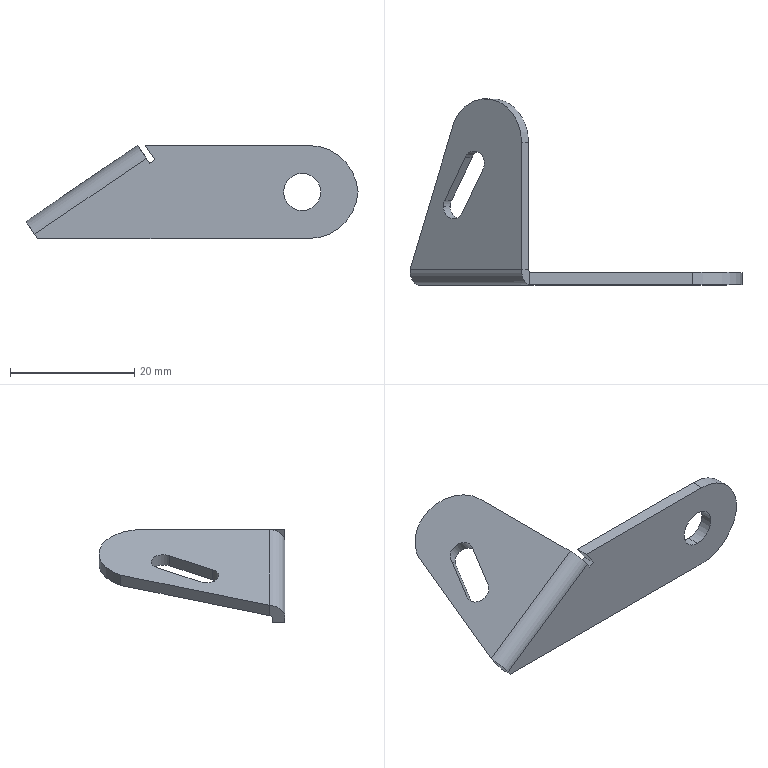Part | SolidWorks | features ICE 3, Cut 2, Fillet 2, EdgeFlange 1, FlatPattern 1, SMBaseFlange 1, SheetMetal 1 | 1 solid | 25 faces | box 53.504 x 30 x 15 mm | volume 2061 mm3 | plane 15 | cylinder 10 | commonest cylinder face diameters 4 x3 6 x2 16 x2 1 x1 5 x1 14 x1
STEP:
#1=CARTESIAN_POINT('',(-11.933,11.65,-0.9332));
#2=VERTEX_POINT('',#1);
#3=CARTESIAN_POINT('',(-12.155,10.65,-1.084));
#4=VERTEX_POINT('',#3);
#5=CARTESIAN_POINT('',(-10.501,10.65,0.04121));
#6=DIRECTION('',(-0.5626,0.,0.8267));
#7=DIRECTION('',(0.8267,0.,0.5626));
#8=AXIS2_PLACEMENT_3D('',#5,#6,#7);
#9=CIRCLE('',#8,2.);
#10=EDGE_CURVE('',#2,#4,#9,.T.);
#11=ORIENTED_EDGE('',*,*,#10,.T.);
#12=CARTESIAN_POINT('',(-11.03,10.65,-2.737));
#13=VERTEX_POINT('',#12);
#14=CARTESIAN_POINT('',(-16.655,10.65,5.53));
#15=DIRECTION('',(0.5626,0.,-0.8267));
#16=VECTOR('',#15,1000.);
#17=LINE('',#14,#16);
#18=EDGE_CURVE('',#4,#13,#17,.T.);
#19=ORIENTED_EDGE('',*,*,#18,.T.);
#20=CARTESIAN_POINT('',(-10.808,11.65,-2.587));
#21=VERTEX_POINT('',#20);
#22=CARTESIAN_POINT('',(-9.376,10.65,-1.612));
#23=DIRECTION('',(0.5626,0.,-0.8267));
#24=DIRECTION('',(-0.8267,0.,-0.5626));
#25=AXIS2_PLACEMENT_3D('',#22,#23,#24);
#26=CIRCLE('',#25,2.);
#27=EDGE_CURVE('',#13,#21,#26,.T.);
#28=ORIENTED_EDGE('',*,*,#27,.T.);
#29=CARTESIAN_POINT('',(-16.434,11.65,5.681));
#30=DIRECTION('',(0.5626,0.,-0.8267));
#31=VECTOR('',#30,1000.);
#32=LINE('',#29,#31);
#33=EDGE_CURVE('',#2,#21,#32,.T.);
#34=ORIENTED_EDGE('',*,*,#33,.F.);
#35=EDGE_LOOP('',(#11,#19,#28,#34));
#36=FACE_OUTER_BOUND('',#35,.T.);
#37=CARTESIAN_POINT('',(-15.002,10.65,6.655));
#38=DIRECTION('',(0.5626,0.,-0.8267));
#39=DIRECTION('',(-0.8267,0.,-0.5626));
#40=AXIS2_PLACEMENT_3D('',#37,#38,#39);
#41=CYLINDRICAL_SURFACE('',#40,2.);
#42=ADVANCED_FACE('',(#36),#41,.F.);
#43=CARTESIAN_POINT('',(27.,-2.,-3.));
#44=VERTEX_POINT('',#43);
#45=CARTESIAN_POINT('',(27.,-2.,3.));
#46=VERTEX_POINT('',#45);
#47=CARTESIAN_POINT('',(27.,-2.,0.));
#48=DIRECTION('',(0.,1.,0.));
#49=DIRECTION('',(0.,0.,1.));
#50=AXIS2_PLACEMENT_3D('',#47,#48,#49);
#51=CIRCLE('',#50,3.);
#52=EDGE_CURVE('',#44,#46,#51,.T.);
#53=ORIENTED_EDGE('',*,*,#52,.F.);
#54=CARTESIAN_POINT('',(27.,0.,-3.));
#55=VERTEX_POINT('',#54);
#56=CARTESIAN_POINT('',(27.,-2.,-3.));
#57=DIRECTION('',(0.,1.,0.));
#58=VECTOR('',#57,1000.);
#59=LINE('',#56,#58);
#60=EDGE_CURVE('',#44,#55,#59,.T.);
#61=ORIENTED_EDGE('',*,*,#60,.T.);
#62=CARTESIAN_POINT('',(27.,0.,3.));
#63=VERTEX_POINT('',#62);
#64=CARTESIAN_POINT('',(27.,0.,0.));
#65=DIRECTION('',(0.,1.,0.));
#66=DIRECTION('',(0.,0.,1.));
#67=AXIS2_PLACEMENT_3D('',#64,#65,#66);
#68=CIRCLE('',#67,3.);
#69=EDGE_CURVE('',#55,#63,#68,.T.);
#70=ORIENTED_EDGE('',*,*,#69,.T.);
#71=CARTESIAN_POINT('',(27.,-2.,3.));
#72=DIRECTION('',(0.,1.,0.));
#73=VECTOR('',#72,1000.);
#74=LINE('',#71,#73);
#75=EDGE_CURVE('',#46,#63,#74,.T.);
#76=ORIENTED_EDGE('',*,*,#75,.F.);
#77=EDGE_LOOP('',(#53,#61,#70,#76));
#78=FACE_OUTER_BOUND('',#77,.T.);
#79=CARTESIAN_POINT('',(27.,-2.,0.));
#80=DIRECTION('',(0.,1.,0.));
#81=DIRECTION('',(0.,0.,1.));
#82=AXIS2_PLACEMENT_3D('',#79,#80,#81);
#83=CYLINDRICAL_SURFACE('',#82,3.);
#84=ADVANCED_FACE('',(#78),#83,.F.);
#85=CARTESIAN_POINT('',(1.669,-2.,7.5));
#86=VERTEX_POINT('',#85);
#87=CARTESIAN_POINT('',(28.,-2.,7.5));
#88=VERTEX_POINT('',#87);
#89=CARTESIAN_POINT('',(-36.,-2.,7.5));
#90=DIRECTION('',(1.,0.,0.));
#91=VECTOR('',#90,1000.);
#92=LINE('',#89,#91);
#93=EDGE_CURVE('',#86,#88,#92,.T.);
#94=ORIENTED_EDGE('',*,*,#93,.T.);
#95=CARTESIAN_POINT('',(28.,0.,7.5));
#96=VERTEX_POINT('',#95);
#97=CARTESIAN_POINT('',(28.,-2.,7.5));
#98=DIRECTION('',(0.,1.,0.));
#99=VECTOR('',#98,1000.);
#100=LINE('',#97,#99);
#101=EDGE_CURVE('',#88,#96,#100,.T.);
#102=ORIENTED_EDGE('',*,*,#101,.T.);
#103=CARTESIAN_POINT('',(1.669,0.,7.5));
#104=VERTEX_POINT('',#103);
#105=CARTESIAN_POINT('',(-36.,0.,7.5));
#106=DIRECTION('',(1.,0.,0.));
#107=VECTOR('',#106,1000.);
#108=LINE('',#105,#107);
#109=EDGE_CURVE('',#104,#96,#108,.T.);
#110=ORIENTED_EDGE('',*,*,#109,.F.);
#111=CARTESIAN_POINT('',(1.669,0.,7.5));
#112=DIRECTION('',(0.,-1.,0.));
#113=VECTOR('',#112,1000.);
#114=LINE('',#111,#113);
#115=EDGE_CURVE('',#104,#86,#114,.T.);
#116=ORIENTED_EDGE('',*,*,#115,.T.);
#117=EDGE_LOOP('',(#94,#102,#110,#116));
#118=FACE_OUTER_BOUND('',#117,.T.);
#119=CARTESIAN_POINT('',(-36.,-2.,7.5));
#120=DIRECTION('',(0.,0.,1.));
#121=DIRECTION('',(1.,0.,0.));
#122=AXIS2_PLACEMENT_3D('',#119,#120,#121);
#123=PLANE('',#122);
#124=ADVANCED_FACE('',(#118),#123,.T.);
#125=CARTESIAN_POINT('',(-15.638,0.,-7.5));
#126=VERTEX_POINT('',#125);
#127=CARTESIAN_POINT('',(-15.638,-2.,-7.5));
#128=VERTEX_POINT('',#127);
#129=CARTESIAN_POINT('',(-15.638,-2.,-7.5));
#130=DIRECTION('',(0.,-1.,0.));
#131=VECTOR('',#130,1000.);
#132=LINE('',#129,#131);
#133=EDGE_CURVE('',#126,#128,#132,.T.);
#134=ORIENTED_EDGE('',*,*,#133,.F.);
#135=CARTESIAN_POINT('',(28.,0.,-7.5));
#136=VERTEX_POINT('',#135);
#137=CARTESIAN_POINT('',(-36.,0.,-7.5));
#138=DIRECTION('',(-1.,0.,0.));
#139=VECTOR('',#138,1000.);
#140=LINE('',#137,#139);
#141=EDGE_CURVE('',#136,#126,#140,.T.);
#142=ORIENTED_EDGE('',*,*,#141,.F.);
#143=CARTESIAN_POINT('',(28.,-2.,-7.5));
#144=VERTEX_POINT('',#143);
#145=CARTESIAN_POINT('',(28.,-2.,-7.5));
#146=DIRECTION('',(0.,-1.,0.));
#147=VECTOR('',#146,1000.);
#148=LINE('',#145,#147);
#149=EDGE_CURVE('',#136,#144,#148,.T.);
#150=ORIENTED_EDGE('',*,*,#149,.T.);
#151=CARTESIAN_POINT('',(-36.,-2.,-7.5));
#152=DIRECTION('',(-1.,0.,0.));
#153=VECTOR('',#152,1000.);
#154=LINE('',#151,#153);
#155=EDGE_CURVE('',#144,#128,#154,.T.);
#156=ORIENTED_EDGE('',*,*,#155,.T.);
#157=EDGE_LOOP('',(#134,#142,#150,#156));
#158=FACE_OUTER_BOUND('',#157,.T.);
#159=CARTESIAN_POINT('',(-36.,-2.,-7.5));
#160=DIRECTION('',(0.,0.,-1.));
#161=DIRECTION('',(-1.,0.,0.));
#162=AXIS2_PLACEMENT_3D('',#159,#160,#161);
#163=PLANE('',#162);
#164=ADVANCED_FACE('',(#158),#163,.T.);
#165=CARTESIAN_POINT('',(27.,-2.,0.));
#166=DIRECTION('',(0.,1.,0.));
#167=DIRECTION('',(0.,0.,1.));
#168=AXIS2_PLACEMENT_3D('',#165,#166,#167);
#169=CIRCLE('',#168,3.);
#170=EDGE_CURVE('',#46,#44,#169,.T.);
#171=ORIENTED_EDGE('',*,*,#170,.T.);
#172=ORIENTED_EDGE('',*,*,#52,.T.);
#173=EDGE_LOOP('',(#171,#172));
#174=FACE_BOUND('',#173,.T.);
#175=CARTESIAN_POINT('',(1.866,-2.,5.433));
#176=VERTEX_POINT('',#175);
#177=CARTESIAN_POINT('',(-16.113,-2.,-6.802));
#178=VERTEX_POINT('',#177);
#179=CARTESIAN_POINT('',(1.866,-2.,5.433));
#180=DIRECTION('',(-0.8267,0.,-0.5626));
#181=VECTOR('',#180,1000.);
#182=LINE('',#179,#181);
#183=EDGE_CURVE('',#176,#178,#182,.T.);
#184=ORIENTED_EDGE('',*,*,#183,.T.);
#185=CARTESIAN_POINT('',(-14.177,-2.,-9.647));
#186=DIRECTION('',(0.5626,0.,-0.8267));
#187=VECTOR('',#186,1000.);
#188=LINE('',#185,#187);
#189=EDGE_CURVE('',#178,#128,#188,.T.);
#190=ORIENTED_EDGE('',*,*,#189,.T.);
#191=ORIENTED_EDGE('',*,*,#155,.F.);
#192=CARTESIAN_POINT('',(35.984,-2.,0.));
#193=VERTEX_POINT('',#192);
#194=CARTESIAN_POINT('',(28.,-2.,0.5));
#195=DIRECTION('',(0.,-1.,0.));
#196=DIRECTION('',(0.,0.,1.));
#197=AXIS2_PLACEMENT_3D('',#194,#195,#196);
#198=CIRCLE('',#197,8.);
#199=EDGE_CURVE('',#144,#193,#198,.T.);
#200=ORIENTED_EDGE('',*,*,#199,.T.);
#201=CARTESIAN_POINT('',(28.,-2.,-0.5));
#202=DIRECTION('',(0.,-1.,0.));
#203=DIRECTION('',(0.,0.,1.));
#204=AXIS2_PLACEMENT_3D('',#201,#202,#203);
#205=CIRCLE('',#204,8.);
#206=EDGE_CURVE('',#193,#88,#205,.T.);
#207=ORIENTED_EDGE('',*,*,#206,.T.);
#208=ORIENTED_EDGE('',*,*,#93,.F.);
#209=CARTESIAN_POINT('',(3.256,-2.,5.169));
#210=VERTEX_POINT('',#209);
#211=CARTESIAN_POINT('',(4.629,-2.,3.15));
#212=DIRECTION('',(-0.5626,0.,0.8267));
#213=VECTOR('',#212,1000.);
#214=LINE('',#211,#213);
#215=EDGE_CURVE('',#210,#86,#214,.T.);
#216=ORIENTED_EDGE('',*,*,#215,.F.);
#217=CARTESIAN_POINT('',(2.429,-2.,4.606));
#218=VERTEX_POINT('',#217);
#219=CARTESIAN_POINT('',(-1.374,-2.,2.019));
#220=DIRECTION('',(0.8267,0.,0.5626));
#221=VECTOR('',#220,1000.);
#222=LINE('',#219,#221);
#223=EDGE_CURVE('',#218,#210,#222,.T.);
#224=ORIENTED_EDGE('',*,*,#223,.F.);
#225=CARTESIAN_POINT('',(3.803,-2.,2.588));
#226=DIRECTION('',(0.5626,0.,-0.8267));
#227=VECTOR('',#226,1000.);
#228=LINE('',#225,#227);
#229=EDGE_CURVE('',#176,#218,#228,.T.);
#230=ORIENTED_EDGE('',*,*,#229,.F.);
#231=EDGE_LOOP('',(#184,#190,#191,#200,#207,#208,#216,#224,#230));
#232=FACE_OUTER_BOUND('',#231,.T.);
#233=CARTESIAN_POINT('',(0.,-2.,0.));
#234=DIRECTION('',(0.,1.,0.));
#235=DIRECTION('',(0.,0.,1.));
#236=AXIS2_PLACEMENT_3D('',#233,#234,#235);
#237=PLANE('',#236);
#238=ADVANCED_FACE('',(#174,#232),#237,.F.);
#239=CARTESIAN_POINT('',(-16.113,0.,-6.802));
#240=VERTEX_POINT('',#239);
#241=CARTESIAN_POINT('',(-14.177,0.,-9.647));
#242=DIRECTION('',(0.5626,0.,-0.8267));
#243=VECTOR('',#242,1000.);
#244=LINE('',#241,#243);
#245=EDGE_CURVE('',#240,#126,#244,.T.);
#246=ORIENTED_EDGE('',*,*,#245,.F.);
#247=CARTESIAN_POINT('',(1.866,0.,5.433));
#248=VERTEX_POINT('',#247);
#249=CARTESIAN_POINT('',(1.866,0.,5.433));
#250=DIRECTION('',(-0.8267,0.,-0.5626));
#251=VECTOR('',#250,1000.);
#252=LINE('',#249,#251);
#253=EDGE_CURVE('',#248,#240,#252,.T.);
#254=ORIENTED_EDGE('',*,*,#253,.F.);
#255=CARTESIAN_POINT('',(2.429,0.,4.606));
#256=VERTEX_POINT('',#255);
#257=CARTESIAN_POINT('',(2.429,0.,4.606));
#258=DIRECTION('',(-0.5626,0.,0.8267));
#259=VECTOR('',#258,1000.);
#260=LINE('',#257,#259);
#261=EDGE_CURVE('',#256,#248,#260,.T.);
#262=ORIENTED_EDGE('',*,*,#261,.F.);
#263=CARTESIAN_POINT('',(3.256,0.,5.169));
#264=VERTEX_POINT('',#263);
#265=CARTESIAN_POINT('',(3.256,0.,5.169));
#266=DIRECTION('',(-0.8267,0.,-0.5626));
#267=VECTOR('',#266,1000.);
#268=LINE('',#265,#267);
#269=EDGE_CURVE('',#264,#256,#268,.T.);
#270=ORIENTED_EDGE('',*,*,#269,.F.);
#271=CARTESIAN_POINT('',(1.669,0.,7.5));
#272=DIRECTION('',(0.5626,0.,-0.8267));
#273=VECTOR('',#272,1000.);
#274=LINE('',#271,#273);
#275=EDGE_CURVE('',#104,#264,#274,.T.);
#276=ORIENTED_EDGE('',*,*,#275,.F.);
#277=ORIENTED_EDGE('',*,*,#109,.T.);
#278=CARTESIAN_POINT('',(35.984,0.,0.));
#279=VERTEX_POINT('',#278);
#280=CARTESIAN_POINT('',(28.,0.,-0.5));
#281=DIRECTION('',(0.,1.,0.));
#282=DIRECTION('',(0.,0.,1.));
#283=AXIS2_PLACEMENT_3D('',#280,#281,#282);
#284=CIRCLE('',#283,8.);
#285=EDGE_CURVE('',#96,#279,#284,.T.);
#286=ORIENTED_EDGE('',*,*,#285,.T.);
#287=CARTESIAN_POINT('',(28.,0.,0.5));
#288=DIRECTION('',(0.,1.,0.));
#289=DIRECTION('',(0.,0.,1.));
#290=AXIS2_PLACEMENT_3D('',#287,#288,#289);
#291=CIRCLE('',#290,8.);
#292=EDGE_CURVE('',#279,#136,#291,.T.);
#293=ORIENTED_EDGE('',*,*,#292,.T.);
#294=ORIENTED_EDGE('',*,*,#141,.T.);
#295=EDGE_LOOP('',(#246,#254,#262,#270,#276,#277,#286,#293,#294));
#296=FACE_OUTER_BOUND('',#295,.T.);
#297=CARTESIAN_POINT('',(27.,0.,0.));
#298=DIRECTION('',(0.,1.,0.));
#299=DIRECTION('',(0.,0.,1.));
#300=AXIS2_PLACEMENT_3D('',#297,#298,#299);
#301=CIRCLE('',#300,3.);
#302=EDGE_CURVE('',#63,#55,#301,.T.);
#303=ORIENTED_EDGE('',*,*,#302,.F.);
#304=ORIENTED_EDGE('',*,*,#69,.F.);
#305=EDGE_LOOP('',(#303,#304));
#306=FACE_BOUND('',#305,.T.);
#307=CARTESIAN_POINT('',(0.,0.,0.));
#308=DIRECTION('',(0.,1.,0.));
#309=DIRECTION('',(0.,0.,1.));
#310=AXIS2_PLACEMENT_3D('',#307,#308,#309);
#311=PLANE('',#310);
#312=ADVANCED_FACE('',(#296,#306),#311,.T.);
#313=ORIENTED_EDGE('',*,*,#60,.F.);
#314=ORIENTED_EDGE('',*,*,#170,.F.);
#315=ORIENTED_EDGE('',*,*,#75,.T.);
#316=ORIENTED_EDGE('',*,*,#302,.T.);
#317=EDGE_LOOP('',(#313,#314,#315,#316));
#318=FACE_OUTER_BOUND('',#317,.T.);
#319=CARTESIAN_POINT('',(27.,-2.,0.));
#320=DIRECTION('',(0.,1.,0.));
#321=DIRECTION('',(0.,0.,1.));
#322=AXIS2_PLACEMENT_3D('',#319,#320,#321);
#323=CYLINDRICAL_SURFACE('',#322,3.);
#324=ADVANCED_FACE('',(#318),#323,.F.);
#325=CARTESIAN_POINT('',(3.256,0.,5.169));
#326=DIRECTION('',(0.,-1.,0.));
#327=VECTOR('',#326,1000.);
#328=LINE('',#325,#327);
#329=EDGE_CURVE('',#264,#210,#328,.T.);
#330=ORIENTED_EDGE('',*,*,#329,.T.);
#331=ORIENTED_EDGE('',*,*,#215,.T.);
#332=ORIENTED_EDGE('',*,*,#115,.F.);
#333=ORIENTED_EDGE('',*,*,#275,.T.);
#334=EDGE_LOOP('',(#330,#331,#332,#333));
#335=FACE_OUTER_BOUND('',#334,.T.);
#336=CARTESIAN_POINT('',(1.669,0.,7.5));
#337=DIRECTION('',(-0.8267,0.,-0.5626));
#338=DIRECTION('',(-0.5626,0.,0.8267));
#339=AXIS2_PLACEMENT_3D('',#336,#337,#338);
#340=PLANE('',#339);
#341=ADVANCED_FACE('',(#335),#340,.T.);
#342=CARTESIAN_POINT('',(2.429,0.,4.606));
#343=DIRECTION('',(0.,-1.,0.));
#344=VECTOR('',#343,1000.);
#345=LINE('',#342,#344);
#346=EDGE_CURVE('',#256,#218,#345,.T.);
#347=ORIENTED_EDGE('',*,*,#346,.T.);
#348=ORIENTED_EDGE('',*,*,#223,.T.);
#349=ORIENTED_EDGE('',*,*,#329,.F.);
#350=ORIENTED_EDGE('',*,*,#269,.T.);
#351=EDGE_LOOP('',(#347,#348,#349,#350));
#352=FACE_OUTER_BOUND('',#351,.T.);
#353=CARTESIAN_POINT('',(3.256,0.,5.169));
#354=DIRECTION('',(-0.5626,0.,0.8267));
#355=DIRECTION('',(0.8267,0.,0.5626));
#356=AXIS2_PLACEMENT_3D('',#353,#354,#355);
#357=PLANE('',#356);
#358=ADVANCED_FACE('',(#352),#357,.T.);
#359=CARTESIAN_POINT('',(1.866,0.,5.433));
#360=DIRECTION('',(0.,-1.,0.));
#361=VECTOR('',#360,1000.);
#362=LINE('',#359,#361);
#363=EDGE_CURVE('',#248,#176,#362,.T.);
#364=ORIENTED_EDGE('',*,*,#363,.T.);
#365=ORIENTED_EDGE('',*,*,#229,.T.);
#366=ORIENTED_EDGE('',*,*,#346,.F.);
#367=ORIENTED_EDGE('',*,*,#261,.T.);
#368=EDGE_LOOP('',(#364,#365,#366,#367));
#369=FACE_OUTER_BOUND('',#368,.T.);
#370=CARTESIAN_POINT('',(2.429,0.,4.606));
#371=DIRECTION('',(0.8267,0.,0.5626));
#372=DIRECTION('',(0.5626,0.,-0.8267));
#373=AXIS2_PLACEMENT_3D('',#370,#371,#372);
#374=PLANE('',#373);
#375=ADVANCED_FACE('',(#369),#374,.T.);
#376=CARTESIAN_POINT('',(1.585,0.5,5.847));
#377=VERTEX_POINT('',#376);
#378=CARTESIAN_POINT('',(1.866,0.5,5.433));
#379=DIRECTION('',(0.8267,0.,0.5626));
#380=DIRECTION('',(0.5626,0.,-0.8267));
#381=AXIS2_PLACEMENT_3D('',#378,#379,#380);
#382=CIRCLE('',#381,0.5);
#383=EDGE_CURVE('',#377,#248,#382,.T.);
#384=ORIENTED_EDGE('',*,*,#383,.F.);
#385=CARTESIAN_POINT('',(0.4598,0.5,7.5));
#386=VERTEX_POINT('',#385);
#387=CARTESIAN_POINT('',(1.585,0.5,5.847));
#388=DIRECTION('',(-0.5626,0.,0.8267));
#389=VECTOR('',#388,1000.);
#390=LINE('',#387,#389);
#391=EDGE_CURVE('',#377,#386,#390,.T.);
#392=ORIENTED_EDGE('',*,*,#391,.T.);
#393=CARTESIAN_POINT('',(1.866,0.5,5.433));
#394=DIRECTION('',(0.8267,0.,0.5626));
#395=DIRECTION('',(0.5626,0.,-0.8267));
#396=AXIS2_PLACEMENT_3D('',#393,#394,#395);
#397=CIRCLE('',#396,2.5);
#398=EDGE_CURVE('',#386,#176,#397,.T.);
#399=ORIENTED_EDGE('',*,*,#398,.T.);
#400=ORIENTED_EDGE('',*,*,#363,.F.);
#401=EDGE_LOOP('',(#384,#392,#399,#400));
#402=FACE_OUTER_BOUND('',#401,.T.);
#403=CARTESIAN_POINT('',(1.866,0.5,5.433));
#404=DIRECTION('',(-0.8267,0.,-0.5626));
#405=DIRECTION('',(-0.5626,0.,0.8267));
#406=AXIS2_PLACEMENT_3D('',#403,#404,#405);
#407=PLANE('',#406);
#408=ADVANCED_FACE('',(#402),#407,.F.);
#409=CARTESIAN_POINT('',(-17.52,0.5,-4.735));
#410=VERTEX_POINT('',#409);
#411=CARTESIAN_POINT('',(-16.113,0.5,-6.802));
#412=DIRECTION('',(-0.8267,0.,-0.5626));
#413=DIRECTION('',(0.5626,0.,-0.8267));
#414=AXIS2_PLACEMENT_3D('',#411,#412,#413);
#415=CIRCLE('',#414,2.5);
#416=EDGE_CURVE('',#178,#410,#415,.T.);
#417=ORIENTED_EDGE('',*,*,#416,.F.);
#418=ORIENTED_EDGE('',*,*,#183,.F.);
#419=ORIENTED_EDGE('',*,*,#398,.F.);
#420=CARTESIAN_POINT('',(-3.343,0.5,4.912));
#421=DIRECTION('',(0.8267,0.,0.5626));
#422=VECTOR('',#421,1000.);
#423=LINE('',#420,#422);
#424=EDGE_CURVE('',#410,#386,#423,.T.);
#425=ORIENTED_EDGE('',*,*,#424,.F.);
#426=EDGE_LOOP('',(#417,#418,#419,#425));
#427=FACE_OUTER_BOUND('',#426,.T.);
#428=CARTESIAN_POINT('',(1.866,0.5,5.433));
#429=DIRECTION('',(0.8267,0.,0.5626));
#430=DIRECTION('',(-0.5626,0.,0.8267));
#431=AXIS2_PLACEMENT_3D('',#428,#429,#430);
#432=CYLINDRICAL_SURFACE('',#431,2.5);
#433=ADVANCED_FACE('',(#427),#432,.T.);
#434=ORIENTED_EDGE('',*,*,#253,.T.);
#435=CARTESIAN_POINT('',(-16.395,0.5,-6.388));
#436=VERTEX_POINT('',#435);
#437=CARTESIAN_POINT('',(-16.113,0.5,-6.802));
#438=DIRECTION('',(-0.8267,0.,-0.5626));
#439=DIRECTION('',(0.5626,0.,-0.8267));
#440=AXIS2_PLACEMENT_3D('',#437,#438,#439);
#441=CIRCLE('',#440,0.5);
#442=EDGE_CURVE('',#240,#436,#441,.T.);
#443=ORIENTED_EDGE('',*,*,#442,.T.);
#444=CARTESIAN_POINT('',(-20.458,0.5,-9.153));
#445=DIRECTION('',(0.8267,0.,0.5626));
#446=VECTOR('',#445,1000.);
#447=LINE('',#444,#446);
#448=EDGE_CURVE('',#436,#377,#447,.T.);
#449=ORIENTED_EDGE('',*,*,#448,.T.);
#450=ORIENTED_EDGE('',*,*,#383,.T.);
#451=EDGE_LOOP('',(#434,#443,#449,#450));
#452=FACE_OUTER_BOUND('',#451,.T.);
#453=CARTESIAN_POINT('',(1.866,0.5,5.433));
#454=DIRECTION('',(0.8267,0.,0.5626));
#455=DIRECTION('',(-0.5626,0.,0.8267));
#456=AXIS2_PLACEMENT_3D('',#453,#454,#455);
#457=CYLINDRICAL_SURFACE('',#456,0.5);
#458=ADVANCED_FACE('',(#452),#457,.F.);
#459=CARTESIAN_POINT('',(1.585,21.,5.847));
#460=VERTEX_POINT('',#459);
#461=CARTESIAN_POINT('',(1.585,0.,5.847));
#462=DIRECTION('',(0.,-1.,0.));
#463=VECTOR('',#462,1000.);
#464=LINE('',#461,#463);
#465=EDGE_CURVE('',#460,#377,#464,.T.);
#466=ORIENTED_EDGE('',*,*,#465,.F.);
#467=CARTESIAN_POINT('',(0.4598,21.,7.5));
#468=VERTEX_POINT('',#467);
#469=CARTESIAN_POINT('',(0.4598,21.,7.5));
#470=DIRECTION('',(-0.5626,0.,0.8267));
#471=VECTOR('',#470,1000.);
#472=LINE('',#469,#471);
#473=EDGE_CURVE('',#460,#468,#472,.T.);
#474=ORIENTED_EDGE('',*,*,#473,.T.);
#475=CARTESIAN_POINT('',(0.4598,0.,7.5));
#476=DIRECTION('',(0.,-1.,0.));
#477=VECTOR('',#476,1000.);
#478=LINE('',#475,#477);
#479=EDGE_CURVE('',#468,#386,#478,.T.);
#480=ORIENTED_EDGE('',*,*,#479,.T.);
#481=ORIENTED_EDGE('',*,*,#391,.F.);
#482=EDGE_LOOP('',(#466,#474,#480,#481));
#483=FACE_OUTER_BOUND('',#482,.T.);
#484=CARTESIAN_POINT('',(0.4598,0.,7.5));
#485=DIRECTION('',(0.8267,0.,0.5626));
#486=DIRECTION('',(0.5626,0.,-0.8267));
#487=AXIS2_PLACEMENT_3D('',#484,#485,#486);
#488=PLANE('',#487);
#489=ADVANCED_FACE('',(#483),#488,.T.);
#490=CARTESIAN_POINT('',(-10.362,24.451,0.1357));
#491=VERTEX_POINT('',#490);
#492=CARTESIAN_POINT('',(-5.327,21.,3.562));
#493=DIRECTION('',(-0.5626,0.,0.8267));
#494=DIRECTION('',(0.8267,0.,0.5626));
#495=AXIS2_PLACEMENT_3D('',#492,#493,#494);
#496=CIRCLE('',#495,7.);
#497=EDGE_CURVE('',#468,#491,#496,.T.);
#498=ORIENTED_EDGE('',*,*,#497,.T.);
#499=CARTESIAN_POINT('',(-16.014,5.54,-3.71));
#500=DIRECTION('',(-0.281,-0.9404,-0.1912));
#501=VECTOR('',#500,1000.);
#502=LINE('',#499,#501);
#503=EDGE_CURVE('',#491,#410,#502,.T.);
#504=ORIENTED_EDGE('',*,*,#503,.T.);
#505=ORIENTED_EDGE('',*,*,#424,.T.);
#506=ORIENTED_EDGE('',*,*,#479,.F.);
#507=EDGE_LOOP('',(#498,#504,#505,#506));
#508=FACE_OUTER_BOUND('',#507,.T.);
#509=CARTESIAN_POINT('',(-5.762,16.578,3.266));
#510=VERTEX_POINT('',#509);
#511=CARTESIAN_POINT('',(-8.626,18.578,1.317));
#512=VERTEX_POINT('',#511);
#513=CARTESIAN_POINT('',(-7.194,17.578,2.292));
#514=DIRECTION('',(-0.5626,0.,0.8267));
#515=DIRECTION('',(0.8267,0.,0.5626));
#516=AXIS2_PLACEMENT_3D('',#513,#514,#515);
#517=CIRCLE('',#516,2.);
#518=EDGE_CURVE('',#510,#512,#517,.T.);
#519=ORIENTED_EDGE('',*,*,#518,.F.);
#520=CARTESIAN_POINT('',(-9.069,9.65,1.016));
#521=VERTEX_POINT('',#520);
#522=CARTESIAN_POINT('',(-11.092,5.412,-0.3609));
#523=DIRECTION('',(0.4134,0.866,0.2813));
#524=VECTOR('',#523,1000.);
#525=LINE('',#522,#524);
#526=EDGE_CURVE('',#521,#510,#525,.T.);
#527=ORIENTED_EDGE('',*,*,#526,.F.);
#528=CARTESIAN_POINT('',(-10.501,10.65,0.04121));
#529=DIRECTION('',(-0.5626,0.,0.8267));
#530=DIRECTION('',(0.8267,0.,0.5626));
#531=AXIS2_PLACEMENT_3D('',#528,#529,#530);
#532=CIRCLE('',#531,2.);
#533=EDGE_CURVE('',#4,#521,#532,.T.);
#534=ORIENTED_EDGE('',*,*,#533,.F.);
#535=ORIENTED_EDGE('',*,*,#10,.F.);
#536=CARTESIAN_POINT('',(-13.956,7.412,-2.31));
#537=DIRECTION('',(-0.4134,-0.866,-0.2813));
#538=VECTOR('',#537,1000.);
#539=LINE('',#536,#538);
#540=EDGE_CURVE('',#512,#2,#539,.T.);
#541=ORIENTED_EDGE('',*,*,#540,.F.);
#542=EDGE_LOOP('',(#519,#527,#534,#535,#541));
#543=FACE_BOUND('',#542,.T.);
#544=CARTESIAN_POINT('',(-3.343,0.,4.912));
#545=DIRECTION('',(-0.5626,0.,0.8267));
#546=DIRECTION('',(0.8267,0.,0.5626));
#547=AXIS2_PLACEMENT_3D('',#544,#545,#546);
#548=PLANE('',#547);
#549=ADVANCED_FACE('',(#508,#543),#548,.T.);
#550=CARTESIAN_POINT('',(-4.637,16.578,1.612));
#551=VERTEX_POINT('',#550);
#552=CARTESIAN_POINT('',(-7.944,9.65,-0.6378));
#553=VERTEX_POINT('',#552);
#554=CARTESIAN_POINT('',(-4.637,16.578,1.612));
#555=DIRECTION('',(-0.4134,-0.866,-0.2813));
#556=VECTOR('',#555,1000.);
#557=LINE('',#554,#556);
#558=EDGE_CURVE('',#551,#553,#557,.T.);
#559=ORIENTED_EDGE('',*,*,#558,.F.);
#560=CARTESIAN_POINT('',(-7.501,18.578,-0.3364));
#561=VERTEX_POINT('',#560);
#562=CARTESIAN_POINT('',(-6.069,17.578,0.6381));
#563=DIRECTION('',(0.5626,0.,-0.8267));
#564=DIRECTION('',(-0.8267,0.,-0.5626));
#565=AXIS2_PLACEMENT_3D('',#562,#563,#564);
#566=CIRCLE('',#565,2.);
#567=EDGE_CURVE('',#561,#551,#566,.T.);
#568=ORIENTED_EDGE('',*,*,#567,.F.);
#569=CARTESIAN_POINT('',(-7.501,18.578,-0.3364));
#570=DIRECTION('',(0.4134,0.866,0.2813));
#571=VECTOR('',#570,1000.);
#572=LINE('',#569,#571);
#573=EDGE_CURVE('',#21,#561,#572,.T.);
#574=ORIENTED_EDGE('',*,*,#573,.F.);
#575=ORIENTED_EDGE('',*,*,#27,.F.);
#576=CARTESIAN_POINT('',(-9.376,10.65,-1.612));
#577=DIRECTION('',(0.5626,0.,-0.8267));
#578=DIRECTION('',(-0.8267,0.,-0.5626));
#579=AXIS2_PLACEMENT_3D('',#576,#577,#578);
#580=CIRCLE('',#579,2.);
#581=EDGE_CURVE('',#553,#13,#580,.T.);
#582=ORIENTED_EDGE('',*,*,#581,.F.);
#583=EDGE_LOOP('',(#559,#568,#574,#575,#582));
#584=FACE_BOUND('',#583,.T.);
#585=CARTESIAN_POINT('',(-9.237,24.451,-1.518));
#586=VERTEX_POINT('',#585);
#587=CARTESIAN_POINT('',(-14.888,5.54,-5.363));
#588=DIRECTION('',(-0.281,-0.9404,-0.1912));
#589=VECTOR('',#588,1000.);
#590=LINE('',#587,#589);
#591=EDGE_CURVE('',#586,#436,#590,.T.);
#592=ORIENTED_EDGE('',*,*,#591,.F.);
#593=CARTESIAN_POINT('',(-4.202,21.,1.908));
#594=DIRECTION('',(0.5626,0.,-0.8267));
#595=DIRECTION('',(0.8267,0.,0.5626));
#596=AXIS2_PLACEMENT_3D('',#593,#594,#595);
#597=CIRCLE('',#596,7.);
#598=EDGE_CURVE('',#586,#460,#597,.T.);
#599=ORIENTED_EDGE('',*,*,#598,.T.);
#600=ORIENTED_EDGE('',*,*,#465,.T.);
#601=ORIENTED_EDGE('',*,*,#448,.F.);
#602=EDGE_LOOP('',(#592,#599,#600,#601));
#603=FACE_OUTER_BOUND('',#602,.T.);
#604=CARTESIAN_POINT('',(-2.218,0.,3.259));
#605=DIRECTION('',(-0.5626,0.,0.8267));
#606=DIRECTION('',(0.8267,0.,0.5626));
#607=AXIS2_PLACEMENT_3D('',#604,#605,#606);
#608=PLANE('',#607);
#609=ADVANCED_FACE('',(#584,#603),#608,.F.);
#610=ORIENTED_EDGE('',*,*,#101,.F.);
#611=ORIENTED_EDGE('',*,*,#206,.F.);
#612=CARTESIAN_POINT('',(35.984,-1.,0.));
#613=DIRECTION('',(0.,-1.,0.));
#614=VECTOR('',#613,1000.);
#615=LINE('',#612,#614);
#616=EDGE_CURVE('',#279,#193,#615,.T.);
#617=ORIENTED_EDGE('',*,*,#616,.F.);
#618=ORIENTED_EDGE('',*,*,#285,.F.);
#619=EDGE_LOOP('',(#610,#611,#617,#618));
#620=FACE_OUTER_BOUND('',#619,.T.);
#621=CARTESIAN_POINT('',(28.,-2.,-0.5));
#622=DIRECTION('',(0.,1.,0.));
#623=DIRECTION('',(0.,0.,1.));
#624=AXIS2_PLACEMENT_3D('',#621,#622,#623);
#625=CYLINDRICAL_SURFACE('',#624,8.);
#626=ADVANCED_FACE('',(#620),#625,.T.);
#627=ORIENTED_EDGE('',*,*,#199,.F.);
#628=ORIENTED_EDGE('',*,*,#149,.F.);
#629=ORIENTED_EDGE('',*,*,#292,.F.);
#630=ORIENTED_EDGE('',*,*,#616,.T.);
#631=EDGE_LOOP('',(#627,#628,#629,#630));
#632=FACE_OUTER_BOUND('',#631,.T.);
#633=CARTESIAN_POINT('',(28.,-2.,0.5));
#634=DIRECTION('',(0.,1.,0.));
#635=DIRECTION('',(0.,0.,1.));
#636=AXIS2_PLACEMENT_3D('',#633,#634,#635);
#637=CYLINDRICAL_SURFACE('',#636,8.);
#638=ADVANCED_FACE('',(#632),#637,.T.);
#639=ORIENTED_EDGE('',*,*,#497,.F.);
#640=ORIENTED_EDGE('',*,*,#473,.F.);
#641=ORIENTED_EDGE('',*,*,#598,.F.);
#642=CARTESIAN_POINT('',(8.627,24.451,-27.77));
#643=DIRECTION('',(-0.5626,0.,0.8267));
#644=VECTOR('',#643,1000.);
#645=LINE('',#642,#644);
#646=EDGE_CURVE('',#586,#491,#645,.T.);
#647=ORIENTED_EDGE('',*,*,#646,.T.);
#648=EDGE_LOOP('',(#639,#640,#641,#647));
#649=FACE_OUTER_BOUND('',#648,.T.);
#650=CARTESIAN_POINT('',(-5.327,21.,3.562));
#651=DIRECTION('',(0.5626,0.,-0.8267));
#652=DIRECTION('',(-0.8267,0.,-0.5626));
#653=AXIS2_PLACEMENT_3D('',#650,#651,#652);
#654=CYLINDRICAL_SURFACE('',#653,7.);
#655=ADVANCED_FACE('',(#649),#654,.T.);
#656=ORIENTED_EDGE('',*,*,#518,.T.);
#657=CARTESIAN_POINT('',(-13.127,18.578,7.931));
#658=DIRECTION('',(0.5626,0.,-0.8267));
#659=VECTOR('',#658,1000.);
#660=LINE('',#657,#659);
#661=EDGE_CURVE('',#512,#561,#660,.T.);
#662=ORIENTED_EDGE('',*,*,#661,.T.);
#663=ORIENTED_EDGE('',*,*,#567,.T.);
#664=CARTESIAN_POINT('',(-10.263,16.578,9.88));
#665=DIRECTION('',(0.5626,0.,-0.8267));
#666=VECTOR('',#665,1000.);
#667=LINE('',#664,#666);
#668=EDGE_CURVE('',#510,#551,#667,.T.);
#669=ORIENTED_EDGE('',*,*,#668,.F.);
#670=EDGE_LOOP('',(#656,#662,#663,#669));
#671=FACE_OUTER_BOUND('',#670,.T.);
#672=CARTESIAN_POINT('',(-11.695,17.578,8.905));
#673=DIRECTION('',(0.5626,0.,-0.8267));
#674=DIRECTION('',(-0.8267,0.,-0.5626));
#675=AXIS2_PLACEMENT_3D('',#672,#673,#674);
#676=CYLINDRICAL_SURFACE('',#675,2.);
#677=ADVANCED_FACE('',(#671),#676,.F.);
#678=ORIENTED_EDGE('',*,*,#540,.T.);
#679=ORIENTED_EDGE('',*,*,#33,.T.);
#680=ORIENTED_EDGE('',*,*,#573,.T.);
#681=ORIENTED_EDGE('',*,*,#661,.F.);
#682=EDGE_LOOP('',(#678,#679,#680,#681));
#683=FACE_OUTER_BOUND('',#682,.T.);
#684=CARTESIAN_POINT('',(-13.127,18.578,7.931));
#685=DIRECTION('',(-0.716,0.5,-0.4872));
#686=DIRECTION('',(-0.5726,-0.8199,0.));
#687=AXIS2_PLACEMENT_3D('',#684,#685,#686);
#688=PLANE('',#687);
#689=ADVANCED_FACE('',(#683),#688,.F.);
#690=ORIENTED_EDGE('',*,*,#18,.F.);
#691=ORIENTED_EDGE('',*,*,#533,.T.);
#692=CARTESIAN_POINT('',(-13.57,9.65,7.63));
#693=DIRECTION('',(0.5626,0.,-0.8267));
#694=VECTOR('',#693,1000.);
#695=LINE('',#692,#694);
#696=EDGE_CURVE('',#521,#553,#695,.T.);
#697=ORIENTED_EDGE('',*,*,#696,.T.);
#698=ORIENTED_EDGE('',*,*,#581,.T.);
#699=EDGE_LOOP('',(#690,#691,#697,#698));
#700=FACE_OUTER_BOUND('',#699,.T.);
#701=CARTESIAN_POINT('',(-15.002,10.65,6.655));
#702=DIRECTION('',(0.5626,0.,-0.8267));
#703=DIRECTION('',(-0.8267,0.,-0.5626));
#704=AXIS2_PLACEMENT_3D('',#701,#702,#703);
#705=CYLINDRICAL_SURFACE('',#704,2.);
#706=ADVANCED_FACE('',(#700),#705,.F.);
#707=ORIENTED_EDGE('',*,*,#526,.T.);
#708=ORIENTED_EDGE('',*,*,#668,.T.);
#709=ORIENTED_EDGE('',*,*,#558,.T.);
#710=ORIENTED_EDGE('',*,*,#696,.F.);
#711=EDGE_LOOP('',(#707,#708,#709,#710));
#712=FACE_OUTER_BOUND('',#711,.T.);
#713=CARTESIAN_POINT('',(-10.263,16.578,9.88));
#714=DIRECTION('',(0.716,-0.5,0.4872));
#715=DIRECTION('',(0.5726,0.8199,0.));
#716=AXIS2_PLACEMENT_3D('',#713,#714,#715);
#717=PLANE('',#716);
#718=ADVANCED_FACE('',(#712),#717,.F.);
#719=ORIENTED_EDGE('',*,*,#646,.F.);
#720=ORIENTED_EDGE('',*,*,#591,.T.);
#721=CARTESIAN_POINT('',(1.469,0.5,-32.64));
#722=DIRECTION('',(-0.5626,0.,0.8267));
#723=VECTOR('',#722,1000.);
#724=LINE('',#721,#723);
#725=EDGE_CURVE('',#436,#410,#724,.T.);
#726=ORIENTED_EDGE('',*,*,#725,.T.);
#727=ORIENTED_EDGE('',*,*,#503,.F.);
#728=EDGE_LOOP('',(#719,#720,#726,#727));
#729=FACE_OUTER_BOUND('',#728,.T.);
#730=CARTESIAN_POINT('',(2.976,5.54,-31.615));
#731=DIRECTION('',(-0.7775,0.3399,-0.5291));
#732=DIRECTION('',(-0.5626,0.,0.8267));
#733=AXIS2_PLACEMENT_3D('',#730,#731,#732);
#734=PLANE('',#733);
#735=ADVANCED_FACE('',(#729),#734,.T.);
#736=ORIENTED_EDGE('',*,*,#416,.T.);
#737=ORIENTED_EDGE('',*,*,#725,.F.);
#738=ORIENTED_EDGE('',*,*,#442,.F.);
#739=ORIENTED_EDGE('',*,*,#245,.T.);
#740=ORIENTED_EDGE('',*,*,#133,.T.);
#741=ORIENTED_EDGE('',*,*,#189,.F.);
#742=EDGE_LOOP('',(#736,#737,#738,#739,#740,#741));
#743=FACE_OUTER_BOUND('',#742,.T.);
#744=CARTESIAN_POINT('',(-16.395,-9.5,-6.388));
#745=DIRECTION('',(0.8267,0.,0.5626));
#746=DIRECTION('',(0.5626,0.,-0.8267));
#747=AXIS2_PLACEMENT_3D('',#744,#745,#746);
#748=PLANE('',#747);
#749=ADVANCED_FACE('',(#743),#748,.F.);
#750=CLOSED_SHELL('',(#42,#84,#124,#164,#238,#312,#324,#341,#358,#375,#408,#433,#458,#489,#549,#609,#626,#638,#655,#677,#689,#706,#718,#735,#749));
#751=MANIFOLD_SOLID_BREP('',#750);
#752=CARTESIAN_POINT('',(0.,0.,0.));
#753=DIRECTION('',(0.,0.,1.));
#754=DIRECTION('',(1.,0.,0.));
#755=AXIS2_PLACEMENT_3D('',#752,#753,#754);
#756=(LENGTH_UNIT()NAMED_UNIT(*)SI_UNIT(.MILLI.,.METRE.));
#757=UNCERTAINTY_MEASURE_WITH_UNIT(LENGTH_MEASURE(0.00001),#756,'','');
#758=(NAMED_UNIT(*)PLANE_ANGLE_UNIT()SI_UNIT($,.RADIAN.));
#759=(NAMED_UNIT(*)SI_UNIT($,.STERADIAN.)SOLID_ANGLE_UNIT());
#760=(GEOMETRIC_REPRESENTATION_CONTEXT(3)GLOBAL_UNCERTAINTY_ASSIGNED_CONTEXT((#757))GLOBAL_UNIT_ASSIGNED_CONTEXT((#756,#758,#759))REPRESENTATION_CONTEXT('',''));
#761=ADVANCED_BREP_SHAPE_REPRESENTATION('',(#751,#755),#760);